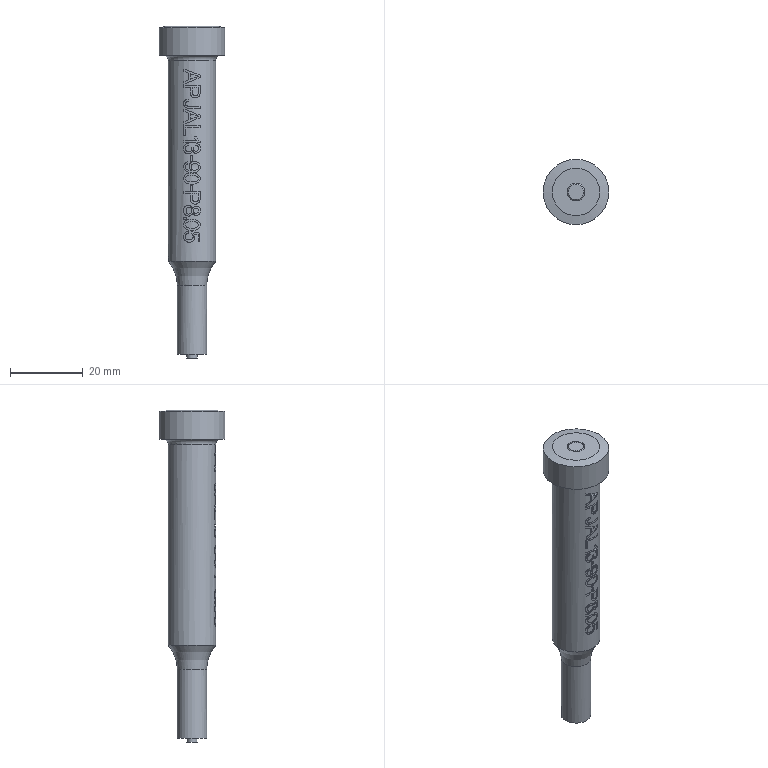Part | NX | features MI_APJAL_0165 2 | 1 solid | 202 faces | box 18 x 18 x 91 mm | volume 10967 mm3 | plane 115 | cylinder 83 | torus 2 | cone 2 | commonest cylinder face diameters 12.8 x16 13 x10 1.447 x2 1.595 x2 1.808 x2 1.894 x2